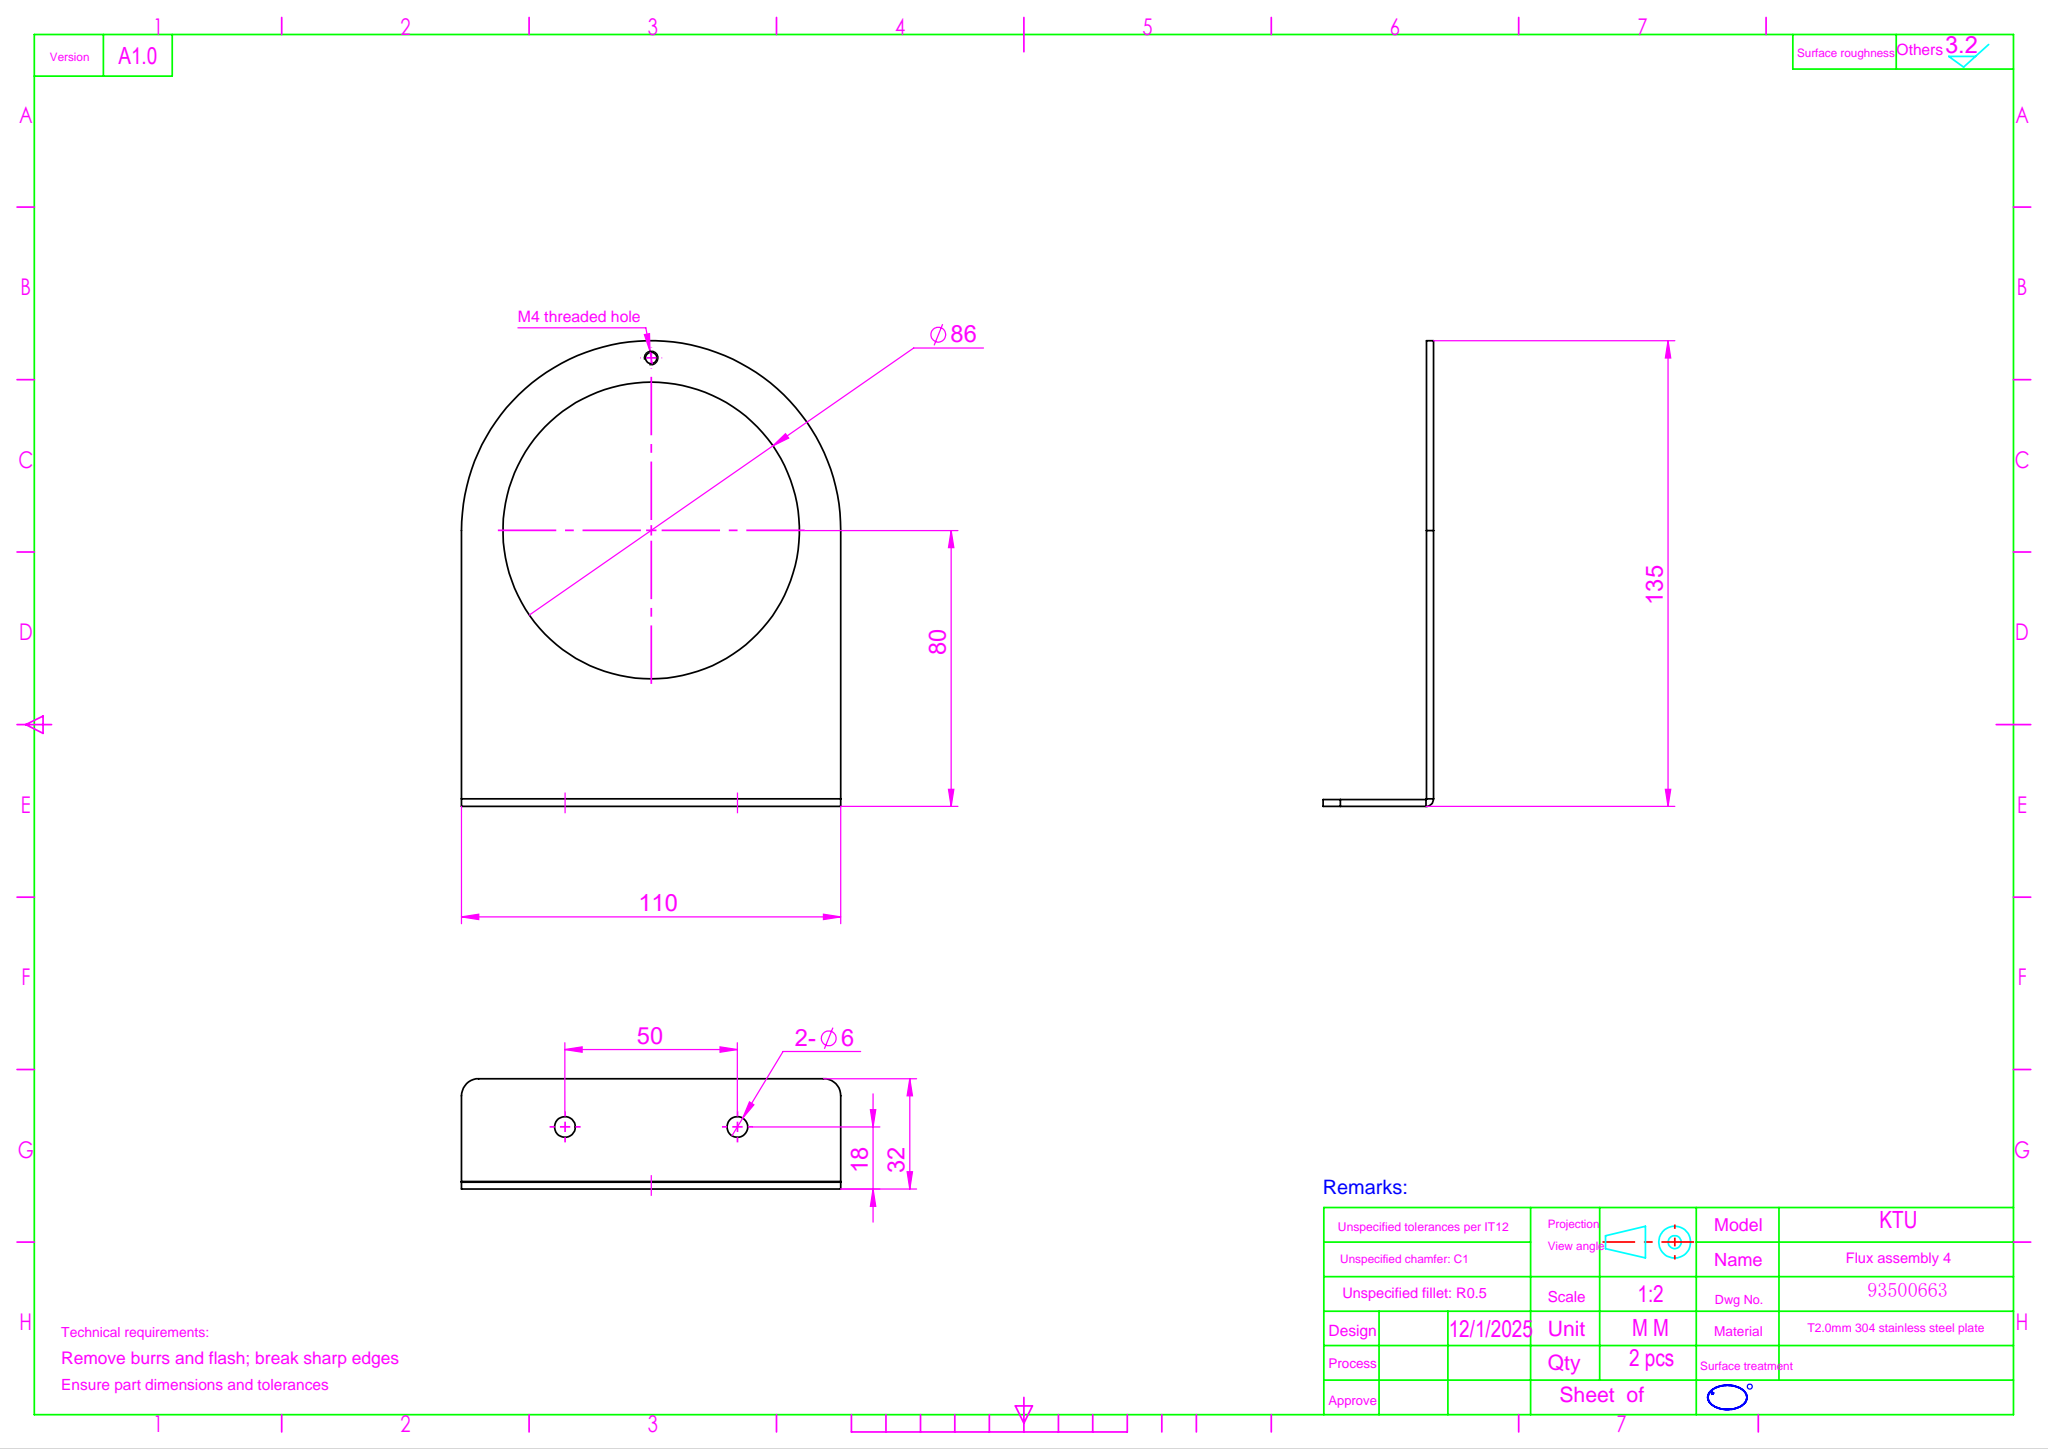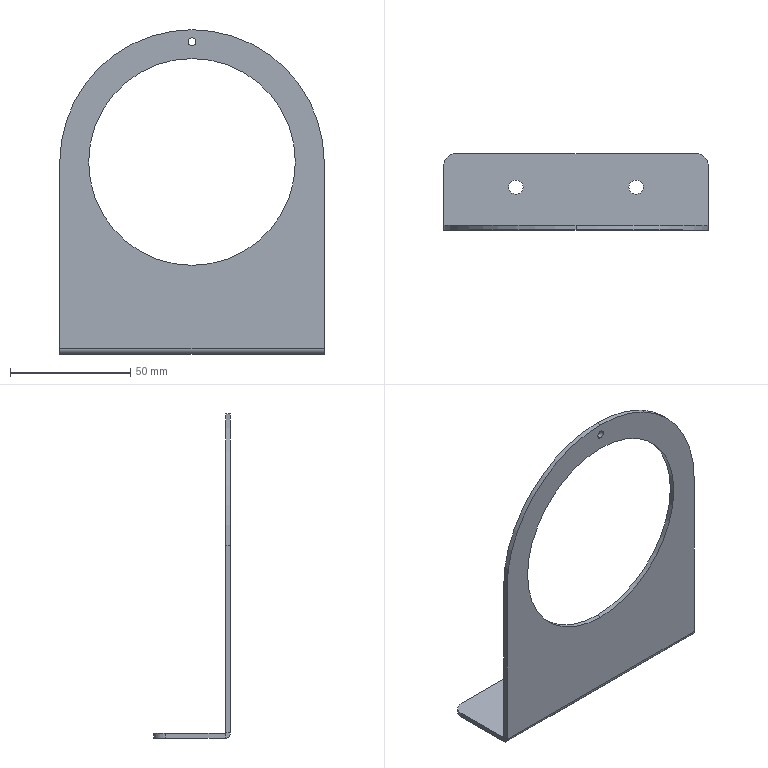Part | SolidWorks | features HoleWzd 2, EdgeFlange 1, Fillet 1, FlatPattern 1, SMBaseFlange 1, SheetMetal 1 | 1 solid | 25 faces | box 110 x 32 x 135 mm | volume 21821 mm3 | cylinder 14 | plane 11 | commonest cylinder face diameters 6 x4 3.3 x2 10 x2 86 x2 110 x2 0.4 x1
STEP:
#1=CARTESIAN_POINT('',(0.,-2.,48.35));
#2=VERTEX_POINT('',#1);
#3=CARTESIAN_POINT('',(0.,-2.,51.65));
#4=VERTEX_POINT('',#3);
#5=CARTESIAN_POINT('',(0.,-2.,50.));
#6=DIRECTION('',(0.,1.,0.));
#7=DIRECTION('',(0.,0.,1.));
#8=AXIS2_PLACEMENT_3D('',#5,#6,#7);
#9=CIRCLE('',#8,1.65);
#10=EDGE_CURVE('',#2,#4,#9,.T.);
#11=ORIENTED_EDGE('',*,*,#10,.F.);
#12=CARTESIAN_POINT('',(0.,0.,48.35));
#13=VERTEX_POINT('',#12);
#14=CARTESIAN_POINT('',(0.,0.,48.35));
#15=DIRECTION('',(0.,1.,0.));
#16=VECTOR('',#15,1000.);
#17=LINE('',#14,#16);
#18=EDGE_CURVE('',#2,#13,#17,.T.);
#19=ORIENTED_EDGE('',*,*,#18,.T.);
#20=CARTESIAN_POINT('',(0.,0.,51.65));
#21=VERTEX_POINT('',#20);
#22=CARTESIAN_POINT('',(0.,0.,50.));
#23=DIRECTION('',(0.,1.,0.));
#24=DIRECTION('',(0.,0.,1.));
#25=AXIS2_PLACEMENT_3D('',#22,#23,#24);
#26=CIRCLE('',#25,1.65);
#27=EDGE_CURVE('',#13,#21,#26,.T.);
#28=ORIENTED_EDGE('',*,*,#27,.T.);
#29=CARTESIAN_POINT('',(0.,0.,51.65));
#30=DIRECTION('',(0.,1.,0.));
#31=VECTOR('',#30,1000.);
#32=LINE('',#29,#31);
#33=EDGE_CURVE('',#4,#21,#32,.T.);
#34=ORIENTED_EDGE('',*,*,#33,.F.);
#35=EDGE_LOOP('',(#11,#19,#28,#34));
#36=FACE_OUTER_BOUND('',#35,.T.);
#37=CARTESIAN_POINT('',(0.,0.,50.));
#38=DIRECTION('',(0.,1.,0.));
#39=DIRECTION('',(0.,0.,1.));
#40=AXIS2_PLACEMENT_3D('',#37,#38,#39);
#41=CYLINDRICAL_SURFACE('',#40,1.65);
#42=ADVANCED_FACE('',(#36),#41,.F.);
#43=CARTESIAN_POINT('',(-28.,16.,-80.));
#44=VERTEX_POINT('',#43);
#45=CARTESIAN_POINT('',(-22.,16.,-80.));
#46=VERTEX_POINT('',#45);
#47=CARTESIAN_POINT('',(-25.,16.,-80.));
#48=DIRECTION('',(0.,0.,1.));
#49=DIRECTION('',(1.,0.,0.));
#50=AXIS2_PLACEMENT_3D('',#47,#48,#49);
#51=CIRCLE('',#50,3.);
#52=EDGE_CURVE('',#44,#46,#51,.T.);
#53=ORIENTED_EDGE('',*,*,#52,.F.);
#54=CARTESIAN_POINT('',(-28.,16.,-78.));
#55=VERTEX_POINT('',#54);
#56=CARTESIAN_POINT('',(-28.,16.,-78.));
#57=DIRECTION('',(0.,0.,1.));
#58=VECTOR('',#57,1000.);
#59=LINE('',#56,#58);
#60=EDGE_CURVE('',#44,#55,#59,.T.);
#61=ORIENTED_EDGE('',*,*,#60,.T.);
#62=CARTESIAN_POINT('',(-22.,16.,-78.));
#63=VERTEX_POINT('',#62);
#64=CARTESIAN_POINT('',(-25.,16.,-78.));
#65=DIRECTION('',(0.,0.,1.));
#66=DIRECTION('',(1.,0.,0.));
#67=AXIS2_PLACEMENT_3D('',#64,#65,#66);
#68=CIRCLE('',#67,3.);
#69=EDGE_CURVE('',#55,#63,#68,.T.);
#70=ORIENTED_EDGE('',*,*,#69,.T.);
#71=CARTESIAN_POINT('',(-22.,16.,-78.));
#72=DIRECTION('',(0.,0.,1.));
#73=VECTOR('',#72,1000.);
#74=LINE('',#71,#73);
#75=EDGE_CURVE('',#46,#63,#74,.T.);
#76=ORIENTED_EDGE('',*,*,#75,.F.);
#77=EDGE_LOOP('',(#53,#61,#70,#76));
#78=FACE_OUTER_BOUND('',#77,.T.);
#79=CARTESIAN_POINT('',(-25.,16.,-78.));
#80=DIRECTION('',(0.,0.,1.));
#81=DIRECTION('',(1.,0.,0.));
#82=AXIS2_PLACEMENT_3D('',#79,#80,#81);
#83=CYLINDRICAL_SURFACE('',#82,3.);
#84=ADVANCED_FACE('',(#78),#83,.F.);
#85=CARTESIAN_POINT('',(22.,16.,-80.));
#86=VERTEX_POINT('',#85);
#87=CARTESIAN_POINT('',(28.,16.,-80.));
#88=VERTEX_POINT('',#87);
#89=CARTESIAN_POINT('',(25.,16.,-80.));
#90=DIRECTION('',(0.,0.,1.));
#91=DIRECTION('',(1.,0.,0.));
#92=AXIS2_PLACEMENT_3D('',#89,#90,#91);
#93=CIRCLE('',#92,3.);
#94=EDGE_CURVE('',#86,#88,#93,.T.);
#95=ORIENTED_EDGE('',*,*,#94,.F.);
#96=CARTESIAN_POINT('',(22.,16.,-78.));
#97=VERTEX_POINT('',#96);
#98=CARTESIAN_POINT('',(22.,16.,-78.));
#99=DIRECTION('',(0.,0.,1.));
#100=VECTOR('',#99,1000.);
#101=LINE('',#98,#100);
#102=EDGE_CURVE('',#86,#97,#101,.T.);
#103=ORIENTED_EDGE('',*,*,#102,.T.);
#104=CARTESIAN_POINT('',(28.,16.,-78.));
#105=VERTEX_POINT('',#104);
#106=CARTESIAN_POINT('',(25.,16.,-78.));
#107=DIRECTION('',(0.,0.,1.));
#108=DIRECTION('',(1.,0.,0.));
#109=AXIS2_PLACEMENT_3D('',#106,#107,#108);
#110=CIRCLE('',#109,3.);
#111=EDGE_CURVE('',#97,#105,#110,.T.);
#112=ORIENTED_EDGE('',*,*,#111,.T.);
#113=CARTESIAN_POINT('',(28.,16.,-78.));
#114=DIRECTION('',(0.,0.,1.));
#115=VECTOR('',#114,1000.);
#116=LINE('',#113,#115);
#117=EDGE_CURVE('',#88,#105,#116,.T.);
#118=ORIENTED_EDGE('',*,*,#117,.F.);
#119=EDGE_LOOP('',(#95,#103,#112,#118));
#120=FACE_OUTER_BOUND('',#119,.T.);
#121=CARTESIAN_POINT('',(25.,16.,-78.));
#122=DIRECTION('',(0.,0.,1.));
#123=DIRECTION('',(1.,0.,0.));
#124=AXIS2_PLACEMENT_3D('',#121,#122,#123);
#125=CYLINDRICAL_SURFACE('',#124,3.);
#126=ADVANCED_FACE('',(#120),#125,.F.);
#127=CARTESIAN_POINT('',(0.,-2.,-43.));
#128=VERTEX_POINT('',#127);
#129=CARTESIAN_POINT('',(0.,-2.,43.));
#130=VERTEX_POINT('',#129);
#131=CARTESIAN_POINT('',(0.,-2.,0.));
#132=DIRECTION('',(0.,1.,0.));
#133=DIRECTION('',(0.,0.,1.));
#134=AXIS2_PLACEMENT_3D('',#131,#132,#133);
#135=CIRCLE('',#134,43.);
#136=EDGE_CURVE('',#128,#130,#135,.T.);
#137=ORIENTED_EDGE('',*,*,#136,.F.);
#138=CARTESIAN_POINT('',(0.,0.,-43.));
#139=VERTEX_POINT('',#138);
#140=CARTESIAN_POINT('',(0.,-2.,-43.));
#141=DIRECTION('',(0.,1.,0.));
#142=VECTOR('',#141,1000.);
#143=LINE('',#140,#142);
#144=EDGE_CURVE('',#128,#139,#143,.T.);
#145=ORIENTED_EDGE('',*,*,#144,.T.);
#146=CARTESIAN_POINT('',(0.,0.,43.));
#147=VERTEX_POINT('',#146);
#148=CARTESIAN_POINT('',(0.,0.,0.));
#149=DIRECTION('',(0.,1.,0.));
#150=DIRECTION('',(0.,0.,1.));
#151=AXIS2_PLACEMENT_3D('',#148,#149,#150);
#152=CIRCLE('',#151,43.);
#153=EDGE_CURVE('',#139,#147,#152,.T.);
#154=ORIENTED_EDGE('',*,*,#153,.T.);
#155=CARTESIAN_POINT('',(0.,-2.,43.));
#156=DIRECTION('',(0.,1.,0.));
#157=VECTOR('',#156,1000.);
#158=LINE('',#155,#157);
#159=EDGE_CURVE('',#130,#147,#158,.T.);
#160=ORIENTED_EDGE('',*,*,#159,.F.);
#161=EDGE_LOOP('',(#137,#145,#154,#160));
#162=FACE_OUTER_BOUND('',#161,.T.);
#163=CARTESIAN_POINT('',(0.,-2.,0.));
#164=DIRECTION('',(0.,1.,0.));
#165=DIRECTION('',(0.,0.,1.));
#166=AXIS2_PLACEMENT_3D('',#163,#164,#165);
#167=CYLINDRICAL_SURFACE('',#166,43.);
#168=ADVANCED_FACE('',(#162),#167,.F.);
#169=CARTESIAN_POINT('',(-55.,-2.,0.));
#170=VERTEX_POINT('',#169);
#171=CARTESIAN_POINT('',(0.,-2.,55.));
#172=VERTEX_POINT('',#171);
#173=CARTESIAN_POINT('',(0.,-2.,0.));
#174=DIRECTION('',(0.,1.,0.));
#175=DIRECTION('',(0.,0.,1.));
#176=AXIS2_PLACEMENT_3D('',#173,#174,#175);
#177=CIRCLE('',#176,55.);
#178=EDGE_CURVE('',#170,#172,#177,.T.);
#179=ORIENTED_EDGE('',*,*,#178,.T.);
#180=CARTESIAN_POINT('',(0.,0.,55.));
#181=VERTEX_POINT('',#180);
#182=CARTESIAN_POINT('',(0.,-2.,55.));
#183=DIRECTION('',(0.,1.,0.));
#184=VECTOR('',#183,1000.);
#185=LINE('',#182,#184);
#186=EDGE_CURVE('',#172,#181,#185,.T.);
#187=ORIENTED_EDGE('',*,*,#186,.T.);
#188=CARTESIAN_POINT('',(-55.,0.,0.));
#189=VERTEX_POINT('',#188);
#190=CARTESIAN_POINT('',(0.,0.,0.));
#191=DIRECTION('',(0.,1.,0.));
#192=DIRECTION('',(0.,0.,1.));
#193=AXIS2_PLACEMENT_3D('',#190,#191,#192);
#194=CIRCLE('',#193,55.);
#195=EDGE_CURVE('',#189,#181,#194,.T.);
#196=ORIENTED_EDGE('',*,*,#195,.F.);
#197=CARTESIAN_POINT('',(-55.,-2.,0.));
#198=DIRECTION('',(0.,1.,0.));
#199=VECTOR('',#198,1000.);
#200=LINE('',#197,#199);
#201=EDGE_CURVE('',#170,#189,#200,.T.);
#202=ORIENTED_EDGE('',*,*,#201,.F.);
#203=EDGE_LOOP('',(#179,#187,#196,#202));
#204=FACE_OUTER_BOUND('',#203,.T.);
#205=CARTESIAN_POINT('',(0.,-2.,0.));
#206=DIRECTION('',(0.,1.,0.));
#207=DIRECTION('',(0.,0.,1.));
#208=AXIS2_PLACEMENT_3D('',#205,#206,#207);
#209=CYLINDRICAL_SURFACE('',#208,55.);
#210=ADVANCED_FACE('',(#204),#209,.T.);
#211=CARTESIAN_POINT('',(-55.,0.,-77.8));
#212=VERTEX_POINT('',#211);
#213=CARTESIAN_POINT('',(-55.,0.,0.));
#214=DIRECTION('',(0.,0.,1.));
#215=VECTOR('',#214,1000.);
#216=LINE('',#213,#215);
#217=EDGE_CURVE('',#212,#189,#216,.T.);
#218=ORIENTED_EDGE('',*,*,#217,.F.);
#219=CARTESIAN_POINT('',(-55.,-2.,-77.8));
#220=VERTEX_POINT('',#219);
#221=CARTESIAN_POINT('',(-55.,0.,-77.8));
#222=DIRECTION('',(0.,-1.,0.));
#223=VECTOR('',#222,1000.);
#224=LINE('',#221,#223);
#225=EDGE_CURVE('',#212,#220,#224,.T.);
#226=ORIENTED_EDGE('',*,*,#225,.T.);
#227=CARTESIAN_POINT('',(-55.,-2.,0.));
#228=DIRECTION('',(0.,0.,1.));
#229=VECTOR('',#228,1000.);
#230=LINE('',#227,#229);
#231=EDGE_CURVE('',#220,#170,#230,.T.);
#232=ORIENTED_EDGE('',*,*,#231,.T.);
#233=ORIENTED_EDGE('',*,*,#201,.T.);
#234=EDGE_LOOP('',(#218,#226,#232,#233));
#235=FACE_OUTER_BOUND('',#234,.T.);
#236=CARTESIAN_POINT('',(-55.,-2.,0.));
#237=DIRECTION('',(-1.,0.,0.));
#238=DIRECTION('',(0.,0.,1.));
#239=AXIS2_PLACEMENT_3D('',#236,#237,#238);
#240=PLANE('',#239);
#241=ADVANCED_FACE('',(#235),#240,.T.);
#242=CARTESIAN_POINT('',(0.,-2.,50.));
#243=DIRECTION('',(0.,1.,0.));
#244=DIRECTION('',(0.,0.,1.));
#245=AXIS2_PLACEMENT_3D('',#242,#243,#244);
#246=CIRCLE('',#245,1.65);
#247=EDGE_CURVE('',#4,#2,#246,.T.);
#248=ORIENTED_EDGE('',*,*,#247,.T.);
#249=ORIENTED_EDGE('',*,*,#10,.T.);
#250=EDGE_LOOP('',(#248,#249));
#251=FACE_BOUND('',#250,.T.);
#252=CARTESIAN_POINT('',(0.,-2.,0.));
#253=DIRECTION('',(0.,1.,0.));
#254=DIRECTION('',(0.,0.,1.));
#255=AXIS2_PLACEMENT_3D('',#252,#253,#254);
#256=CIRCLE('',#255,43.);
#257=EDGE_CURVE('',#130,#128,#256,.T.);
#258=ORIENTED_EDGE('',*,*,#257,.T.);
#259=ORIENTED_EDGE('',*,*,#136,.T.);
#260=EDGE_LOOP('',(#258,#259));
#261=FACE_BOUND('',#260,.T.);
#262=CARTESIAN_POINT('',(55.,-2.,-77.8));
#263=VERTEX_POINT('',#262);
#264=CARTESIAN_POINT('',(-55.,-2.,-77.8));
#265=DIRECTION('',(1.,0.,0.));
#266=VECTOR('',#265,1000.);
#267=LINE('',#264,#266);
#268=EDGE_CURVE('',#220,#263,#267,.T.);
#269=ORIENTED_EDGE('',*,*,#268,.T.);
#270=CARTESIAN_POINT('',(55.,-2.,0.));
#271=VERTEX_POINT('',#270);
#272=CARTESIAN_POINT('',(55.,-2.,-80.));
#273=DIRECTION('',(0.,0.,-1.));
#274=VECTOR('',#273,1000.);
#275=LINE('',#272,#274);
#276=EDGE_CURVE('',#271,#263,#275,.T.);
#277=ORIENTED_EDGE('',*,*,#276,.F.);
#278=CARTESIAN_POINT('',(0.,-2.,0.));
#279=DIRECTION('',(0.,1.,0.));
#280=DIRECTION('',(0.,0.,1.));
#281=AXIS2_PLACEMENT_3D('',#278,#279,#280);
#282=CIRCLE('',#281,55.);
#283=EDGE_CURVE('',#172,#271,#282,.T.);
#284=ORIENTED_EDGE('',*,*,#283,.F.);
#285=ORIENTED_EDGE('',*,*,#178,.F.);
#286=ORIENTED_EDGE('',*,*,#231,.F.);
#287=EDGE_LOOP('',(#269,#277,#284,#285,#286));
#288=FACE_OUTER_BOUND('',#287,.T.);
#289=CARTESIAN_POINT('',(0.,-2.,0.));
#290=DIRECTION('',(0.,1.,0.));
#291=DIRECTION('',(0.,0.,1.));
#292=AXIS2_PLACEMENT_3D('',#289,#290,#291);
#293=PLANE('',#292);
#294=ADVANCED_FACE('',(#251,#261,#288),#293,.F.);
#295=CARTESIAN_POINT('',(0.,0.,50.));
#296=DIRECTION('',(0.,1.,0.));
#297=DIRECTION('',(0.,0.,1.));
#298=AXIS2_PLACEMENT_3D('',#295,#296,#297);
#299=CIRCLE('',#298,1.65);
#300=EDGE_CURVE('',#21,#13,#299,.T.);
#301=ORIENTED_EDGE('',*,*,#300,.F.);
#302=ORIENTED_EDGE('',*,*,#27,.F.);
#303=EDGE_LOOP('',(#301,#302));
#304=FACE_BOUND('',#303,.T.);
#305=CARTESIAN_POINT('',(0.,0.,0.));
#306=DIRECTION('',(0.,1.,0.));
#307=DIRECTION('',(0.,0.,1.));
#308=AXIS2_PLACEMENT_3D('',#305,#306,#307);
#309=CIRCLE('',#308,43.);
#310=EDGE_CURVE('',#147,#139,#309,.T.);
#311=ORIENTED_EDGE('',*,*,#310,.F.);
#312=ORIENTED_EDGE('',*,*,#153,.F.);
#313=EDGE_LOOP('',(#311,#312));
#314=FACE_BOUND('',#313,.T.);
#315=CARTESIAN_POINT('',(55.,0.,0.));
#316=VERTEX_POINT('',#315);
#317=CARTESIAN_POINT('',(55.,0.,-77.8));
#318=VERTEX_POINT('',#317);
#319=CARTESIAN_POINT('',(55.,0.,-80.));
#320=DIRECTION('',(0.,0.,-1.));
#321=VECTOR('',#320,1000.);
#322=LINE('',#319,#321);
#323=EDGE_CURVE('',#316,#318,#322,.T.);
#324=ORIENTED_EDGE('',*,*,#323,.T.);
#325=CARTESIAN_POINT('',(-55.,0.,-77.8));
#326=DIRECTION('',(1.,0.,0.));
#327=VECTOR('',#326,1000.);
#328=LINE('',#325,#327);
#329=EDGE_CURVE('',#212,#318,#328,.T.);
#330=ORIENTED_EDGE('',*,*,#329,.F.);
#331=ORIENTED_EDGE('',*,*,#217,.T.);
#332=ORIENTED_EDGE('',*,*,#195,.T.);
#333=CARTESIAN_POINT('',(0.,0.,0.));
#334=DIRECTION('',(0.,1.,0.));
#335=DIRECTION('',(0.,0.,1.));
#336=AXIS2_PLACEMENT_3D('',#333,#334,#335);
#337=CIRCLE('',#336,55.);
#338=EDGE_CURVE('',#181,#316,#337,.T.);
#339=ORIENTED_EDGE('',*,*,#338,.T.);
#340=EDGE_LOOP('',(#324,#330,#331,#332,#339));
#341=FACE_OUTER_BOUND('',#340,.T.);
#342=CARTESIAN_POINT('',(0.,0.,0.));
#343=DIRECTION('',(0.,1.,0.));
#344=DIRECTION('',(0.,0.,1.));
#345=AXIS2_PLACEMENT_3D('',#342,#343,#344);
#346=PLANE('',#345);
#347=ADVANCED_FACE('',(#304,#314,#341),#346,.T.);
#348=ORIENTED_EDGE('',*,*,#186,.F.);
#349=ORIENTED_EDGE('',*,*,#283,.T.);
#350=CARTESIAN_POINT('',(55.,-2.,0.));
#351=DIRECTION('',(0.,1.,0.));
#352=VECTOR('',#351,1000.);
#353=LINE('',#350,#352);
#354=EDGE_CURVE('',#271,#316,#353,.T.);
#355=ORIENTED_EDGE('',*,*,#354,.T.);
#356=ORIENTED_EDGE('',*,*,#338,.F.);
#357=EDGE_LOOP('',(#348,#349,#355,#356));
#358=FACE_OUTER_BOUND('',#357,.T.);
#359=CARTESIAN_POINT('',(0.,-2.,0.));
#360=DIRECTION('',(0.,1.,0.));
#361=DIRECTION('',(0.,0.,1.));
#362=AXIS2_PLACEMENT_3D('',#359,#360,#361);
#363=CYLINDRICAL_SURFACE('',#362,55.);
#364=ADVANCED_FACE('',(#358),#363,.T.);
#365=CARTESIAN_POINT('',(55.,0.,-77.8));
#366=DIRECTION('',(0.,-1.,0.));
#367=VECTOR('',#366,1000.);
#368=LINE('',#365,#367);
#369=EDGE_CURVE('',#318,#263,#368,.T.);
#370=ORIENTED_EDGE('',*,*,#369,.F.);
#371=ORIENTED_EDGE('',*,*,#323,.F.);
#372=ORIENTED_EDGE('',*,*,#354,.F.);
#373=ORIENTED_EDGE('',*,*,#276,.T.);
#374=EDGE_LOOP('',(#370,#371,#372,#373));
#375=FACE_OUTER_BOUND('',#374,.T.);
#376=CARTESIAN_POINT('',(55.,-2.,-80.));
#377=DIRECTION('',(1.,0.,0.));
#378=DIRECTION('',(0.,0.,-1.));
#379=AXIS2_PLACEMENT_3D('',#376,#377,#378);
#380=PLANE('',#379);
#381=ADVANCED_FACE('',(#375),#380,.T.);
#382=ORIENTED_EDGE('',*,*,#144,.F.);
#383=ORIENTED_EDGE('',*,*,#257,.F.);
#384=ORIENTED_EDGE('',*,*,#159,.T.);
#385=ORIENTED_EDGE('',*,*,#310,.T.);
#386=EDGE_LOOP('',(#382,#383,#384,#385));
#387=FACE_OUTER_BOUND('',#386,.T.);
#388=CARTESIAN_POINT('',(0.,-2.,0.));
#389=DIRECTION('',(0.,1.,0.));
#390=DIRECTION('',(0.,0.,1.));
#391=AXIS2_PLACEMENT_3D('',#388,#389,#390);
#392=CYLINDRICAL_SURFACE('',#391,43.);
#393=ADVANCED_FACE('',(#387),#392,.F.);
#394=CARTESIAN_POINT('',(55.,0.2,-78.));
#395=VERTEX_POINT('',#394);
#396=CARTESIAN_POINT('',(55.,0.2,-80.));
#397=VERTEX_POINT('',#396);
#398=CARTESIAN_POINT('',(55.,0.2,-80.));
#399=DIRECTION('',(0.,0.,-1.));
#400=VECTOR('',#399,1000.);
#401=LINE('',#398,#400);
#402=EDGE_CURVE('',#395,#397,#401,.T.);
#403=ORIENTED_EDGE('',*,*,#402,.F.);
#404=CARTESIAN_POINT('',(55.,0.2,-77.8));
#405=DIRECTION('',(1.,0.,0.));
#406=DIRECTION('',(0.,0.,1.));
#407=AXIS2_PLACEMENT_3D('',#404,#405,#406);
#408=CIRCLE('',#407,0.2);
#409=EDGE_CURVE('',#318,#395,#408,.T.);
#410=ORIENTED_EDGE('',*,*,#409,.F.);
#411=ORIENTED_EDGE('',*,*,#369,.T.);
#412=CARTESIAN_POINT('',(55.,0.2,-77.8));
#413=DIRECTION('',(1.,0.,0.));
#414=DIRECTION('',(0.,0.,1.));
#415=AXIS2_PLACEMENT_3D('',#412,#413,#414);
#416=CIRCLE('',#415,2.2);
#417=EDGE_CURVE('',#263,#397,#416,.T.);
#418=ORIENTED_EDGE('',*,*,#417,.T.);
#419=EDGE_LOOP('',(#403,#410,#411,#418));
#420=FACE_OUTER_BOUND('',#419,.T.);
#421=CARTESIAN_POINT('',(55.,0.2,-77.8));
#422=DIRECTION('',(1.,0.,0.));
#423=DIRECTION('',(0.,0.,-1.));
#424=AXIS2_PLACEMENT_3D('',#421,#422,#423);
#425=PLANE('',#424);
#426=ADVANCED_FACE('',(#420),#425,.T.);
#427=CARTESIAN_POINT('',(-55.,0.2,-78.));
#428=VERTEX_POINT('',#427);
#429=CARTESIAN_POINT('',(-55.,0.2,-77.8));
#430=DIRECTION('',(-1.,0.,0.));
#431=DIRECTION('',(0.,0.,1.));
#432=AXIS2_PLACEMENT_3D('',#429,#430,#431);
#433=CIRCLE('',#432,0.2);
#434=EDGE_CURVE('',#428,#212,#433,.T.);
#435=ORIENTED_EDGE('',*,*,#434,.F.);
#436=CARTESIAN_POINT('',(-55.,0.2,-80.));
#437=VERTEX_POINT('',#436);
#438=CARTESIAN_POINT('',(-55.,0.2,-78.));
#439=DIRECTION('',(0.,0.,-1.));
#440=VECTOR('',#439,1000.);
#441=LINE('',#438,#440);
#442=EDGE_CURVE('',#428,#437,#441,.T.);
#443=ORIENTED_EDGE('',*,*,#442,.T.);
#444=CARTESIAN_POINT('',(-55.,0.2,-77.8));
#445=DIRECTION('',(-1.,0.,0.));
#446=DIRECTION('',(0.,0.,1.));
#447=AXIS2_PLACEMENT_3D('',#444,#445,#446);
#448=CIRCLE('',#447,2.2);
#449=EDGE_CURVE('',#437,#220,#448,.T.);
#450=ORIENTED_EDGE('',*,*,#449,.T.);
#451=ORIENTED_EDGE('',*,*,#225,.F.);
#452=EDGE_LOOP('',(#435,#443,#450,#451));
#453=FACE_OUTER_BOUND('',#452,.T.);
#454=CARTESIAN_POINT('',(-55.,0.2,-77.8));
#455=DIRECTION('',(1.,0.,0.));
#456=DIRECTION('',(0.,0.,-1.));
#457=AXIS2_PLACEMENT_3D('',#454,#455,#456);
#458=PLANE('',#457);
#459=ADVANCED_FACE('',(#453),#458,.F.);
#460=ORIENTED_EDGE('',*,*,#268,.F.);
#461=ORIENTED_EDGE('',*,*,#449,.F.);
#462=CARTESIAN_POINT('',(55.,0.2,-80.));
#463=DIRECTION('',(1.,0.,0.));
#464=VECTOR('',#463,1000.);
#465=LINE('',#462,#464);
#466=EDGE_CURVE('',#437,#397,#465,.T.);
#467=ORIENTED_EDGE('',*,*,#466,.T.);
#468=ORIENTED_EDGE('',*,*,#417,.F.);
#469=EDGE_LOOP('',(#460,#461,#467,#468));
#470=FACE_OUTER_BOUND('',#469,.T.);
#471=CARTESIAN_POINT('',(-55.,0.2,-77.8));
#472=DIRECTION('',(-1.,0.,0.));
#473=DIRECTION('',(0.,0.,-1.));
#474=AXIS2_PLACEMENT_3D('',#471,#472,#473);
#475=CYLINDRICAL_SURFACE('',#474,2.2);
#476=ADVANCED_FACE('',(#470),#475,.T.);
#477=ORIENTED_EDGE('',*,*,#329,.T.);
#478=ORIENTED_EDGE('',*,*,#409,.T.);
#479=CARTESIAN_POINT('',(55.,0.2,-78.));
#480=DIRECTION('',(-1.,0.,0.));
#481=VECTOR('',#480,1000.);
#482=LINE('',#479,#481);
#483=EDGE_CURVE('',#395,#428,#482,.T.);
#484=ORIENTED_EDGE('',*,*,#483,.T.);
#485=ORIENTED_EDGE('',*,*,#434,.T.);
#486=EDGE_LOOP('',(#477,#478,#484,#485));
#487=FACE_OUTER_BOUND('',#486,.T.);
#488=CARTESIAN_POINT('',(-55.,0.2,-77.8));
#489=DIRECTION('',(-1.,0.,0.));
#490=DIRECTION('',(0.,0.,-1.));
#491=AXIS2_PLACEMENT_3D('',#488,#489,#490);
#492=CYLINDRICAL_SURFACE('',#491,0.2);
#493=ADVANCED_FACE('',(#487),#492,.F.);
#494=CARTESIAN_POINT('',(55.,25.,-80.));
#495=VERTEX_POINT('',#494);
#496=CARTESIAN_POINT('',(55.,0.,-80.));
#497=DIRECTION('',(0.,-1.,0.));
#498=VECTOR('',#497,1000.);
#499=LINE('',#496,#498);
#500=EDGE_CURVE('',#495,#397,#499,.T.);
#501=ORIENTED_EDGE('',*,*,#500,.F.);
#502=CARTESIAN_POINT('',(55.,25.,-78.));
#503=VERTEX_POINT('',#502);
#504=CARTESIAN_POINT('',(55.,25.,-80.));
#505=DIRECTION('',(0.,0.,1.));
#506=VECTOR('',#505,1000.);
#507=LINE('',#504,#506);
#508=EDGE_CURVE('',#495,#503,#507,.T.);
#509=ORIENTED_EDGE('',*,*,#508,.T.);
#510=CARTESIAN_POINT('',(55.,0.,-78.));
#511=DIRECTION('',(0.,-1.,0.));
#512=VECTOR('',#511,1000.);
#513=LINE('',#510,#512);
#514=EDGE_CURVE('',#503,#395,#513,.T.);
#515=ORIENTED_EDGE('',*,*,#514,.T.);
#516=ORIENTED_EDGE('',*,*,#402,.T.);
#517=EDGE_LOOP('',(#501,#509,#515,#516));
#518=FACE_OUTER_BOUND('',#517,.T.);
#519=CARTESIAN_POINT('',(55.,0.,-80.));
#520=DIRECTION('',(-1.,0.,0.));
#521=DIRECTION('',(0.,0.,1.));
#522=AXIS2_PLACEMENT_3D('',#519,#520,#521);
#523=PLANE('',#522);
#524=ADVANCED_FACE('',(#518),#523,.F.);
#525=CARTESIAN_POINT('',(-55.,25.,-78.));
#526=VERTEX_POINT('',#525);
#527=CARTESIAN_POINT('',(-55.,30.,-78.));
#528=DIRECTION('',(0.,1.,0.));
#529=VECTOR('',#528,1000.);
#530=LINE('',#527,#529);
#531=EDGE_CURVE('',#428,#526,#530,.T.);
#532=ORIENTED_EDGE('',*,*,#531,.T.);
#533=CARTESIAN_POINT('',(-55.,25.,-80.));
#534=VERTEX_POINT('',#533);
#535=CARTESIAN_POINT('',(-55.,25.,-80.));
#536=DIRECTION('',(0.,0.,-1.));
#537=VECTOR('',#536,1000.);
#538=LINE('',#535,#537);
#539=EDGE_CURVE('',#526,#534,#538,.T.);
#540=ORIENTED_EDGE('',*,*,#539,.T.);
#541=CARTESIAN_POINT('',(-55.,0.,-80.));
#542=DIRECTION('',(0.,1.,0.));
#543=VECTOR('',#542,1000.);
#544=LINE('',#541,#543);
#545=EDGE_CURVE('',#437,#534,#544,.T.);
#546=ORIENTED_EDGE('',*,*,#545,.F.);
#547=ORIENTED_EDGE('',*,*,#442,.F.);
#548=EDGE_LOOP('',(#532,#540,#546,#547));
#549=FACE_OUTER_BOUND('',#548,.T.);
#550=CARTESIAN_POINT('',(-55.,30.,-80.));
#551=DIRECTION('',(1.,0.,0.));
#552=DIRECTION('',(0.,1.,0.));
#553=AXIS2_PLACEMENT_3D('',#550,#551,#552);
#554=PLANE('',#553);
#555=ADVANCED_FACE('',(#549),#554,.F.);
#556=CARTESIAN_POINT('',(-25.,16.,-80.));
#557=DIRECTION('',(0.,0.,1.));
#558=DIRECTION('',(1.,0.,0.));
#559=AXIS2_PLACEMENT_3D('',#556,#557,#558);
#560=CIRCLE('',#559,3.);
#561=EDGE_CURVE('',#46,#44,#560,.T.);
#562=ORIENTED_EDGE('',*,*,#561,.T.);
#563=ORIENTED_EDGE('',*,*,#52,.T.);
#564=EDGE_LOOP('',(#562,#563));
#565=FACE_BOUND('',#564,.T.);
#566=CARTESIAN_POINT('',(25.,16.,-80.));
#567=DIRECTION('',(0.,0.,1.));
#568=DIRECTION('',(1.,0.,0.));
#569=AXIS2_PLACEMENT_3D('',#566,#567,#568);
#570=CIRCLE('',#569,3.);
#571=EDGE_CURVE('',#88,#86,#570,.T.);
#572=ORIENTED_EDGE('',*,*,#571,.T.);
#573=ORIENTED_EDGE('',*,*,#94,.T.);
#574=EDGE_LOOP('',(#572,#573));
#575=FACE_BOUND('',#574,.T.);
#576=ORIENTED_EDGE('',*,*,#545,.T.);
#577=CARTESIAN_POINT('',(-50.,30.,-80.));
#578=VERTEX_POINT('',#577);
#579=CARTESIAN_POINT('',(-50.,25.,-80.));
#580=DIRECTION('',(0.,0.,-1.));
#581=DIRECTION('',(0.,-1.,0.));
#582=AXIS2_PLACEMENT_3D('',#579,#580,#581);
#583=CIRCLE('',#582,5.);
#584=EDGE_CURVE('',#534,#578,#583,.T.);
#585=ORIENTED_EDGE('',*,*,#584,.T.);
#586=CARTESIAN_POINT('',(50.,30.,-80.));
#587=VERTEX_POINT('',#586);
#588=CARTESIAN_POINT('',(0.,30.,-80.));
#589=DIRECTION('',(1.,0.,0.));
#590=VECTOR('',#589,1000.);
#591=LINE('',#588,#590);
#592=EDGE_CURVE('',#578,#587,#591,.T.);
#593=ORIENTED_EDGE('',*,*,#592,.T.);
#594=CARTESIAN_POINT('',(50.,25.,-80.));
#595=DIRECTION('',(0.,0.,-1.));
#596=DIRECTION('',(0.,-1.,0.));
#597=AXIS2_PLACEMENT_3D('',#594,#595,#596);
#598=CIRCLE('',#597,5.);
#599=EDGE_CURVE('',#587,#495,#598,.T.);
#600=ORIENTED_EDGE('',*,*,#599,.T.);
#601=ORIENTED_EDGE('',*,*,#500,.T.);
#602=ORIENTED_EDGE('',*,*,#466,.F.);
#603=EDGE_LOOP('',(#576,#585,#593,#600,#601,#602));
#604=FACE_OUTER_BOUND('',#603,.T.);
#605=CARTESIAN_POINT('',(0.,0.,-80.));
#606=DIRECTION('',(0.,0.,1.));
#607=DIRECTION('',(0.,-1.,0.));
#608=AXIS2_PLACEMENT_3D('',#605,#606,#607);
#609=PLANE('',#608);
#610=ADVANCED_FACE('',(#565,#575,#604),#609,.F.);
#611=CARTESIAN_POINT('',(-25.,16.,-78.));
#612=DIRECTION('',(0.,0.,1.));
#613=DIRECTION('',(1.,0.,0.));
#614=AXIS2_PLACEMENT_3D('',#611,#612,#613);
#615=CIRCLE('',#614,3.);
#616=EDGE_CURVE('',#63,#55,#615,.T.);
#617=ORIENTED_EDGE('',*,*,#616,.F.);
#618=ORIENTED_EDGE('',*,*,#69,.F.);
#619=EDGE_LOOP('',(#617,#618));
#620=FACE_BOUND('',#619,.T.);
#621=CARTESIAN_POINT('',(25.,16.,-78.));
#622=DIRECTION('',(0.,0.,1.));
#623=DIRECTION('',(1.,0.,0.));
#624=AXIS2_PLACEMENT_3D('',#621,#622,#623);
#625=CIRCLE('',#624,3.);
#626=EDGE_CURVE('',#105,#97,#625,.T.);
#627=ORIENTED_EDGE('',*,*,#626,.F.);
#628=ORIENTED_EDGE('',*,*,#111,.F.);
#629=EDGE_LOOP('',(#627,#628));
#630=FACE_BOUND('',#629,.T.);
#631=CARTESIAN_POINT('',(-50.,30.,-78.));
#632=VERTEX_POINT('',#631);
#633=CARTESIAN_POINT('',(50.,30.,-78.));
#634=VERTEX_POINT('',#633);
#635=CARTESIAN_POINT('',(55.,30.,-78.));
#636=DIRECTION('',(1.,0.,0.));
#637=VECTOR('',#636,1000.);
#638=LINE('',#635,#637);
#639=EDGE_CURVE('',#632,#634,#638,.T.);
#640=ORIENTED_EDGE('',*,*,#639,.F.);
#641=CARTESIAN_POINT('',(-50.,25.,-78.));
#642=DIRECTION('',(0.,0.,1.));
#643=DIRECTION('',(0.,-1.,0.));
#644=AXIS2_PLACEMENT_3D('',#641,#642,#643);
#645=CIRCLE('',#644,5.);
#646=EDGE_CURVE('',#632,#526,#645,.T.);
#647=ORIENTED_EDGE('',*,*,#646,.T.);
#648=ORIENTED_EDGE('',*,*,#531,.F.);
#649=ORIENTED_EDGE('',*,*,#483,.F.);
#650=ORIENTED_EDGE('',*,*,#514,.F.);
#651=CARTESIAN_POINT('',(50.,25.,-78.));
#652=DIRECTION('',(0.,0.,1.));
#653=DIRECTION('',(0.,-1.,0.));
#654=AXIS2_PLACEMENT_3D('',#651,#652,#653);
#655=CIRCLE('',#654,5.);
#656=EDGE_CURVE('',#503,#634,#655,.T.);
#657=ORIENTED_EDGE('',*,*,#656,.T.);
#658=EDGE_LOOP('',(#640,#647,#648,#649,#650,#657));
#659=FACE_OUTER_BOUND('',#658,.T.);
#660=CARTESIAN_POINT('',(0.,0.,-78.));
#661=DIRECTION('',(0.,0.,1.));
#662=DIRECTION('',(0.,-1.,0.));
#663=AXIS2_PLACEMENT_3D('',#660,#661,#662);
#664=PLANE('',#663);
#665=ADVANCED_FACE('',(#620,#630,#659),#664,.T.);
#666=ORIENTED_EDGE('',*,*,#592,.F.);
#667=CARTESIAN_POINT('',(-50.,30.,-80.));
#668=DIRECTION('',(0.,0.,1.));
#669=VECTOR('',#668,1000.);
#670=LINE('',#667,#669);
#671=EDGE_CURVE('',#578,#632,#670,.T.);
#672=ORIENTED_EDGE('',*,*,#671,.T.);
#673=ORIENTED_EDGE('',*,*,#639,.T.);
#674=CARTESIAN_POINT('',(50.,30.,-80.));
#675=DIRECTION('',(0.,0.,-1.));
#676=VECTOR('',#675,1000.);
#677=LINE('',#674,#676);
#678=EDGE_CURVE('',#634,#587,#677,.T.);
#679=ORIENTED_EDGE('',*,*,#678,.T.);
#680=EDGE_LOOP('',(#666,#672,#673,#679));
#681=FACE_OUTER_BOUND('',#680,.T.);
#682=CARTESIAN_POINT('',(55.,30.,-80.));
#683=DIRECTION('',(0.,-1.,0.));
#684=DIRECTION('',(0.,0.,-1.));
#685=AXIS2_PLACEMENT_3D('',#682,#683,#684);
#686=PLANE('',#685);
#687=ADVANCED_FACE('',(#681),#686,.F.);
#688=ORIENTED_EDGE('',*,*,#102,.F.);
#689=ORIENTED_EDGE('',*,*,#571,.F.);
#690=ORIENTED_EDGE('',*,*,#117,.T.);
#691=ORIENTED_EDGE('',*,*,#626,.T.);
#692=EDGE_LOOP('',(#688,#689,#690,#691));
#693=FACE_OUTER_BOUND('',#692,.T.);
#694=CARTESIAN_POINT('',(25.,16.,-78.));
#695=DIRECTION('',(0.,0.,1.));
#696=DIRECTION('',(1.,0.,0.));
#697=AXIS2_PLACEMENT_3D('',#694,#695,#696);
#698=CYLINDRICAL_SURFACE('',#697,3.);
#699=ADVANCED_FACE('',(#693),#698,.F.);
#700=ORIENTED_EDGE('',*,*,#60,.F.);
#701=ORIENTED_EDGE('',*,*,#561,.F.);
#702=ORIENTED_EDGE('',*,*,#75,.T.);
#703=ORIENTED_EDGE('',*,*,#616,.T.);
#704=EDGE_LOOP('',(#700,#701,#702,#703));
#705=FACE_OUTER_BOUND('',#704,.T.);
#706=CARTESIAN_POINT('',(-25.,16.,-78.));
#707=DIRECTION('',(0.,0.,1.));
#708=DIRECTION('',(1.,0.,0.));
#709=AXIS2_PLACEMENT_3D('',#706,#707,#708);
#710=CYLINDRICAL_SURFACE('',#709,3.);
#711=ADVANCED_FACE('',(#705),#710,.F.);
#712=ORIENTED_EDGE('',*,*,#18,.F.);
#713=ORIENTED_EDGE('',*,*,#247,.F.);
#714=ORIENTED_EDGE('',*,*,#33,.T.);
#715=ORIENTED_EDGE('',*,*,#300,.T.);
#716=EDGE_LOOP('',(#712,#713,#714,#715));
#717=FACE_OUTER_BOUND('',#716,.T.);
#718=CARTESIAN_POINT('',(0.,0.,50.));
#719=DIRECTION('',(0.,1.,0.));
#720=DIRECTION('',(0.,0.,1.));
#721=AXIS2_PLACEMENT_3D('',#718,#719,#720);
#722=CYLINDRICAL_SURFACE('',#721,1.65);
#723=ADVANCED_FACE('',(#717),#722,.F.);
#724=ORIENTED_EDGE('',*,*,#584,.F.);
#725=ORIENTED_EDGE('',*,*,#539,.F.);
#726=ORIENTED_EDGE('',*,*,#646,.F.);
#727=ORIENTED_EDGE('',*,*,#671,.F.);
#728=EDGE_LOOP('',(#724,#725,#726,#727));
#729=FACE_OUTER_BOUND('',#728,.T.);
#730=CARTESIAN_POINT('',(-50.,25.,-80.));
#731=DIRECTION('',(0.,0.,1.));
#732=DIRECTION('',(0.,-1.,0.));
#733=AXIS2_PLACEMENT_3D('',#730,#731,#732);
#734=CYLINDRICAL_SURFACE('',#733,5.);
#735=ADVANCED_FACE('',(#729),#734,.T.);
#736=ORIENTED_EDGE('',*,*,#599,.F.);
#737=ORIENTED_EDGE('',*,*,#678,.F.);
#738=ORIENTED_EDGE('',*,*,#656,.F.);
#739=ORIENTED_EDGE('',*,*,#508,.F.);
#740=EDGE_LOOP('',(#736,#737,#738,#739));
#741=FACE_OUTER_BOUND('',#740,.T.);
#742=CARTESIAN_POINT('',(50.,25.,-80.));
#743=DIRECTION('',(0.,0.,1.));
#744=DIRECTION('',(0.,-1.,0.));
#745=AXIS2_PLACEMENT_3D('',#742,#743,#744);
#746=CYLINDRICAL_SURFACE('',#745,5.);
#747=ADVANCED_FACE('',(#741),#746,.T.);
#748=CLOSED_SHELL('',(#42,#84,#126,#168,#210,#241,#294,#347,#364,#381,#393,#426,#459,#476,#493,#524,#555,#610,#665,#687,#699,#711,#723,#735,#747));
#749=MANIFOLD_SOLID_BREP('',#748);
#750=CARTESIAN_POINT('',(0.,0.,0.));
#751=DIRECTION('',(0.,0.,1.));
#752=DIRECTION('',(1.,0.,0.));
#753=AXIS2_PLACEMENT_3D('',#750,#751,#752);
#754=(LENGTH_UNIT()NAMED_UNIT(*)SI_UNIT(.MILLI.,.METRE.));
#755=UNCERTAINTY_MEASURE_WITH_UNIT(LENGTH_MEASURE(0.00001),#754,'','');
#756=(NAMED_UNIT(*)PLANE_ANGLE_UNIT()SI_UNIT($,.RADIAN.));
#757=(NAMED_UNIT(*)SI_UNIT($,.STERADIAN.)SOLID_ANGLE_UNIT());
#758=(GEOMETRIC_REPRESENTATION_CONTEXT(3)GLOBAL_UNCERTAINTY_ASSIGNED_CONTEXT((#755))GLOBAL_UNIT_ASSIGNED_CONTEXT((#754,#756,#757))REPRESENTATION_CONTEXT('',''));
#759=ADVANCED_BREP_SHAPE_REPRESENTATION('',(#749,#753),#758);